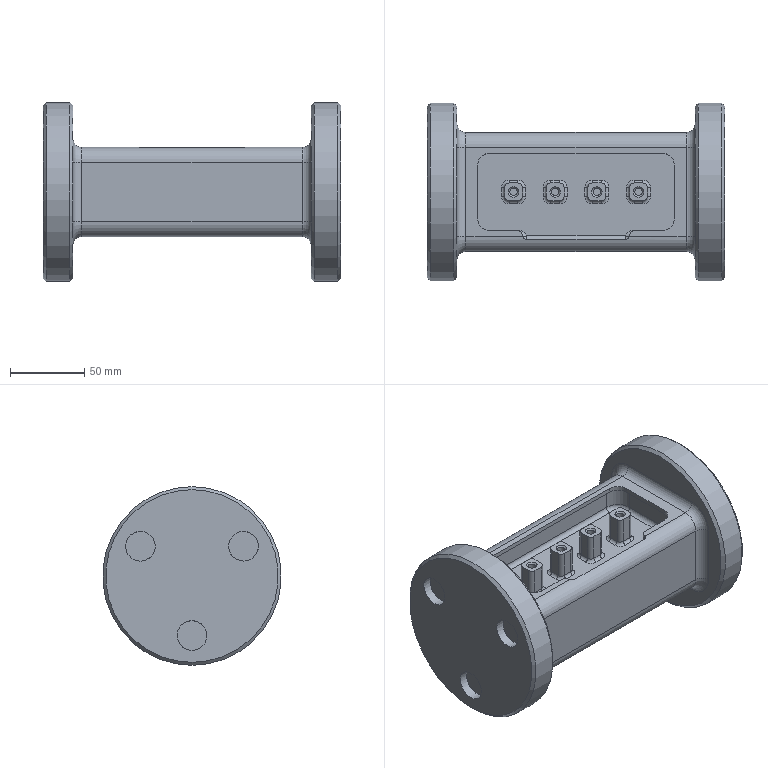NC program | NX | posted with a generic post | part box 200 x 120 x 120 mm
Lines 1229 to 3124 of 4340:
(ZLEVEL_PROFILE , TOOL : D10R1)
N2444 M6
N2446 G53
N2448 G17 G0 G90 X45. Y-16. S0 M3
N2450 G43 Z40. H0
N2452 Z-1.
N2454 G94 G1 Y-14. F250.
N2456 G3 X42. Y-11. R3.
N2458 G1 X39.
N2460 G2 X31. Y-3. R8.
N2462 G1 Y3.
N2464 G2 X39. Y11. R8.
N2466 G1 X45.
N2468 G2 X53. Y3. R8.
N2470 G1 Y-3.
N2472 G2 X45. Y-11. R8.
N2474 G1 X42.
N2476 Z-1.5
N2478 X39.
N2480 G2 X31. Y-3. R8.
N2482 G1 Y3.
N2484 G2 X39. Y11. R8.
N2486 G1 X45.
N2488 G2 X53. Y3. R8.
N2490 G1 Y-3.
N2492 G2 X45. Y-11. R8.
N2494 G1 X42.
N2496 Z-2.
N2498 X39.
N2500 G2 X31. Y-3. R8.
N2502 G1 Y3.
N2504 G2 X39. Y11. R8.
N2506 G1 X45.
N2508 G2 X53. Y3. R8.
N2510 G1 Y-3.
N2512 G2 X45. Y-11. R8.
N2514 G1 X42.
N2516 Z-2.5
N2518 X39.
N2520 G2 X31. Y-3. R8.
N2522 G1 Y3.
N2524 G2 X39. Y11. R8.
N2526 G1 X45.
N2528 G2 X53. Y3. R8.
N2530 G1 Y-3.
N2532 G2 X45. Y-11. R8.
N2534 G1 X42.
N2536 Z-3.
N2538 X39.
N2540 G2 X31. Y-3. R8.
N2542 G1 Y3.
N2544 G2 X39. Y11. R8.
N2546 G1 X45.
N2548 G2 X53. Y3. R8.
N2550 G1 Y-3.
N2552 G2 X45. Y-11. R8.
N2554 G1 X42.
N2556 Z-3.5
N2558 X39.
N2560 G2 X31. Y-3. R8.
N2562 G1 Y3.
N2564 G2 X39. Y11. R8.
N2566 G1 X45.
N2568 G2 X53. Y3. R8.
N2570 G1 Y-3.
N2572 G2 X45. Y-11. R8.
N2574 G1 X42.
N2576 Z-4.
N2578 X39.
N2580 G2 X31. Y-3. R8.
N2582 G1 Y3.
N2584 G2 X39. Y11. R8.
N2586 G1 X45.
N2588 G2 X53. Y3. R8.
N2590 G1 Y-3.
N2592 G2 X45. Y-11. R8.
N2594 G1 X42.
N2596 Z-4.5
N2598 X39.
N2600 G2 X31. Y-3. R8.
N2602 G1 Y3.
N2604 G2 X39. Y11. R8.
N2606 G1 X45.
N2608 G2 X53. Y3. R8.
N2610 G1 Y-3.
N2612 G2 X45. Y-11. R8.
N2614 G1 X42.
N2616 Z-5.
N2618 X39.
N2620 G2 X31. Y-3. R8.
N2622 G1 Y3.
N2624 G2 X39. Y11. R8.
N2626 G1 X45.
N2628 G2 X53. Y3. R8.
N2630 G1 Y-3.
N2632 G2 X45. Y-11. R8.
N2634 G1 X42.
N2636 Z-5.5
N2638 X39.
N2640 G2 X31. Y-3. R8.
N2642 G1 Y3.
N2644 G2 X39. Y11. R8.
N2646 G1 X45.
N2648 G2 X53. Y3. R8.
N2650 G1 Y-3.
N2652 G2 X45. Y-11. R8.
N2654 G1 X42.
N2656 Z-6.
N2658 X39.
N2660 G2 X31. Y-3. R8.
N2662 G1 Y3.
N2664 G2 X39. Y11. R8.
N2666 G1 X45.
N2668 G2 X53. Y3. R8.
N2670 G1 Y-3.
N2672 G2 X45. Y-11. R8.
N2674 G1 X42.
N2676 Z-6.5
N2678 X39.
N2680 G2 X31. Y-3. R8.
N2682 G1 Y3.
N2684 G2 X39. Y11. R8.
N2686 G1 X45.
N2688 G2 X53. Y3. R8.
N2690 G1 Y-3.
N2692 G2 X45. Y-11. R8.
N2694 G1 X42.
N2696 Z-7.
N2698 X39.
N2700 G2 X31. Y-3. R8.
N2702 G1 Y3.
N2704 G2 X39. Y11. R8.
N2706 G1 X45.
N2708 G2 X53. Y3. R8.
N2710 G1 Y-3.
N2712 G2 X45. Y-11. R8.
N2714 G1 X42.
N2716 Z-7.5
N2718 X39.
N2720 G2 X31. Y-3. R8.
N2722 G1 Y3.
N2724 G2 X39. Y11. R8.
N2726 G1 X45.
N2728 G2 X53. Y3. R8.
N2730 G1 Y-3.
N2732 G2 X45. Y-11. R8.
N2734 G1 X42.
N2736 Z-8.
N2738 X39.
N2740 G2 X31. Y-3. R8.
N2742 G1 Y3.
N2744 G2 X39. Y11. R8.
N2746 G1 X45.
N2748 G2 X53. Y3. R8.
N2750 G1 Y-3.
N2752 G2 X45. Y-11. R8.
N2754 G1 X42.
N2756 Z-8.5
N2758 X39.
N2760 G2 X31. Y-3. R8.
N2762 G1 Y3.
N2764 G2 X39. Y11. R8.
N2766 G1 X45.
N2768 G2 X53. Y3. R8.
N2770 G1 Y-3.
N2772 G2 X45. Y-11. R8.
N2774 G1 X42.
N2776 Z-9.
N2778 X39.
N2780 G2 X31. Y-3. R8.
N2782 G1 Y3.
N2784 G2 X39. Y11. R8.
N2786 G1 X45.
N2788 G2 X53. Y3. R8.
N2790 G1 Y-3.
N2792 G2 X45. Y-11. R8.
N2794 G1 X42.
N2796 Z-9.5
N2798 X39.
N2800 G2 X31. Y-3. R8.
N2802 G1 Y3.
N2804 G2 X39. Y11. R8.
N2806 G1 X45.
N2808 G2 X53. Y3. R8.
N2810 G1 Y-3.
N2812 G2 X45. Y-11. R8.
N2814 G1 X42.
N2816 Z-10.
N2818 X39.
N2820 G2 X31. Y-3. R8.
N2822 G1 Y3.
N2824 G2 X39. Y11. R8.
N2826 G1 X45.
N2828 G2 X53. Y3. R8.
N2830 G1 Y-3.
N2832 G2 X45. Y-11. R8.
N2834 G1 X42.
N2836 Z-10.5
N2838 X39.
N2840 G2 X31. Y-3. R8.
N2842 G1 Y3.
N2844 G2 X39. Y11. R8.
N2846 G1 X45.
N2848 G2 X53. Y3. R8.
N2850 G1 Y-3.
N2852 G2 X45. Y-11. R8.
N2854 G1 X42.
N2856 Z-11.
N2858 X39.
N2860 G2 X31. Y-3. R8.
N2862 G1 Y3.
N2864 G2 X39. Y11. R8.
N2866 G1 X45.
N2868 G2 X53. Y3. R8.
N2870 G1 Y-3.
N2872 G2 X45. Y-11. R8.
N2874 G1 X42.
N2876 Z-11.5
N2878 X39.
N2880 G2 X31. Y-3. R8.
N2882 G1 Y3.
N2884 G2 X39. Y11. R8.
N2886 G1 X45.
N2888 G2 X53. Y3. R8.
N2890 G1 Y-3.
N2892 G2 X45. Y-11. R8.
N2894 G1 X42.
N2896 Z-12.
N2898 X39.
N2900 G2 X31. Y-3. R8.
N2902 G1 Y3.
N2904 G2 X39. Y11. R8.
N2906 G1 X45.
N2908 G2 X53. Y3. R8.
N2910 G1 Y-3.
N2912 G2 X45. Y-11. R8.
N2914 G1 X42.
N2916 Z-12.5
N2918 X39.
N2920 G2 X31. Y-3. R8.
N2922 G1 Y3.
N2924 G2 X39. Y11. R8.
N2926 G1 X45.
N2928 G2 X53. Y3. R8.
N2930 G1 Y-3.
N2932 G2 X45. Y-11. R8.
N2934 G1 X42.
N2936 Z-13.
N2938 X39.
N2940 G2 X31. Y-3. R8.
N2942 G1 Y3.
N2944 G2 X39. Y11. R8.
N2946 G1 X45.
N2948 G2 X53. Y3. R8.
N2950 G1 Y-3.
N2952 G2 X45. Y-11. R8.
N2954 G1 X42.
N2956 Z-13.5
N2958 X39.
N2960 G2 X31. Y-3. R8.
N2962 G1 Y3.
N2964 G2 X39. Y11. R8.
N2966 G1 X45.
N2968 G2 X53. Y3. R8.
N2970 G1 Y-3.
N2972 G2 X45. Y-11. R8.
N2974 G1 X42.
N2976 Z-14.
N2978 X39.
N2980 G2 X31. Y-3. R8.
N2982 G1 Y3.
N2984 G2 X39. Y11. R8.
N2986 G1 X45.
N2988 G2 X53. Y3. R8.
N2990 G1 Y-3.
N2992 G2 X45. Y-11. R8.
N2994 G1 X42.
N2996 Z-14.5
N2998 X39.
N3000 G2 X31. Y-3. R8.
N3002 G1 Y3.
N3004 G2 X39. Y11. R8.
N3006 G1 X45.
N3008 G2 X53. Y3. R8.
N3010 G1 Y-3.
N3012 G2 X45. Y-11. R8.
N3014 G1 X42.
N3016 Z-15.
N3018 X39.
N3020 G2 X31. Y-3. R8.
N3022 G1 Y3.
N3024 G2 X39. Y11. R8.
N3026 G1 X45.
N3028 G2 X53. Y3. R8.
N3030 G1 Y-3.
N3032 G2 X45. Y-11. R8.
N3034 G1 X42.
N3036 Z-15.5
N3038 X39.
N3040 G2 X31. Y-3. R8.
N3042 G1 Y3.
N3044 G2 X39. Y11. R8.
N3046 G1 X45.
N3048 G2 X53. Y3. R8.
N3050 G1 Y-3.
N3052 G2 X45. Y-11. R8.
N3054 G1 X42.
N3056 Z-16.
N3058 X39.
N3060 G2 X31. Y-3. R8.
N3062 G1 Y3.
N3064 G2 X39. Y11. R8.
N3066 G1 X45.
N3068 G2 X53. Y3. R8.
N3070 G1 Y-3.
N3072 G2 X45. Y-11. R8.
N3074 G1 X42.
N3076 Z-16.5
N3078 X39.
N3080 G2 X31. Y-3. R8.
N3082 G1 Y3.
N3084 G2 X39. Y11. R8.
N3086 G1 X45.
N3088 G2 X53. Y3. R8.
N3090 G1 Y-3.
N3092 G2 X45. Y-11. R8.
N3094 G1 X42.
N3096 Z-17.
N3098 X39.
N3100 G2 X31. Y-3. R8.
N3102 G1 Y3.
N3104 G2 X39. Y11. R8.
N3106 G1 X45.
N3108 G2 X53. Y3. R8.
N3110 G1 Y-3.
N3112 G2 X45. Y-11. R8.
N3114 G1 X42.
N3116 Z-17.5
N3118 X39.
N3120 G2 X31. Y-3. R8.
N3122 G1 Y3.
N3124 G2 X39. Y11. R8.
N3126 G1 X45.
N3128 G2 X53. Y3. R8.
N3130 G1 Y-3.
N3132 G2 X45. Y-11. R8.
N3134 G1 X42.
N3136 Z-18.
N3138 X39.
N3140 G2 X31. Y-3. R8.
N3142 G1 Y3.
N3144 G2 X39. Y11. R8.
N3146 G1 X45.
N3148 G2 X53. Y3. R8.
N3150 G1 Y-3.
N3152 G2 X45. Y-11. R8.
N3154 G1 X42.
N3156 Z-18.5
N3158 X39.
N3160 G2 X31. Y-3. R8.
N3162 G1 Y3.
N3164 G2 X39. Y11. R8.
N3166 G1 X45.
N3168 G2 X53. Y3. R8.
N3170 G1 Y-3.
N3172 G2 X45. Y-11. R8.
N3174 G1 X42.
N3176 Z-19.
N3178 X39.
N3180 G2 X31. Y-3. R8.
N3182 G1 Y3.
N3184 G2 X39. Y11. R8.
N3186 G1 X45.
N3188 G2 X53. Y3. R8.
N3190 G1 Y-3.
N3192 G2 X45. Y-11. R8.
N3194 G1 X42.
N3196 Y-11.008 Z-19.125
N3198 Y-11.032 Z-19.25
N3200 Y-11.073 Z-19.375
N3202 Y-11.134 Z-19.5
N3204 X39.
N3206 G2 X30.866 Y-3. R8.134
N3208 G1 Y3.
N3210 G2 X39. Y11.134 R8.134
N3212 G1 X45.
N3214 G2 X53.134 Y3. R8.134
N3216 G1 Y-3.
N3218 G2 X45. Y-11.134 R8.134
N3220 G1 X42.
N3222 Y-11.219 Z-19.625
N3224 Y-11.339 Z-19.75
N3226 Y-11.417 Z-19.813
N3228 Y-11.516 Z-19.875
N3230 Y-11.652 Z-19.938
N3232 Y-11.878 Z-20.
N3234 X39.
N3236 G2 X30.122 Y-3. R8.878
N3238 G1 Y3.
N3240 G2 X39. Y11.878 R8.878
N3242 G1 X45.
N3244 G2 X53.878 Y3. R8.878
N3246 G1 Y-3.
N3248 G2 X45. Y-11.878 R8.878
N3250 G1 X42.
N3252 G3 X39. Y-14.878 R3.
N3254 G1 Y-16.878
N3256 G0 Z40.
N3258 X17. Y-16.
N3260 Z-1.
N3262 G1 Y-14.
N3264 G3 X14. Y-11. R3.
N3266 G1 X11.
N3268 G2 X3. Y-3. R8.
N3270 G1 Y3.
N3272 G2 X11. Y11. R8.
N3274 G1 X17.
N3276 G2 X25. Y3. R8.
N3278 G1 Y-3.
N3280 G2 X17. Y-11. R8.
N3282 G1 X14.
N3284 Z-1.5
N3286 X11.
N3288 G2 X3. Y-3. R8.
N3290 G1 Y3.
N3292 G2 X11. Y11. R8.
N3294 G1 X17.
N3296 G2 X25. Y3. R8.
N3298 G1 Y-3.
N3300 G2 X17. Y-11. R8.
N3302 G1 X14.
N3304 Z-2.
N3306 X11.
N3308 G2 X3. Y-3. R8.
N3310 G1 Y3.
N3312 G2 X11. Y11. R8.
N3314 G1 X17.
N3316 G2 X25. Y3. R8.
N3318 G1 Y-3.
N3320 G2 X17. Y-11. R8.
N3322 G1 X14.
N3324 Z-2.5
N3326 X11.
N3328 G2 X3. Y-3. R8.
N3330 G1 Y3.
N3332 G2 X11. Y11. R8.
N3334 G1 X17.
N3336 G2 X25. Y3. R8.
N3338 G1 Y-3.
N3340 G2 X17. Y-11. R8.
N3342 G1 X14.
N3344 Z-3.
N3346 X11.
N3348 G2 X3. Y-3. R8.
N3350 G1 Y3.
N3352 G2 X11. Y11. R8.
N3354 G1 X17.
N3356 G2 X25. Y3. R8.
N3358 G1 Y-3.
N3360 G2 X17. Y-11. R8.
N3362 G1 X14.
N3364 Z-3.5
N3366 X11.
N3368 G2 X3. Y-3. R8.
N3370 G1 Y3.
N3372 G2 X11. Y11. R8.
N3374 G1 X17.
N3376 G2 X25. Y3. R8.
N3378 G1 Y-3.
N3380 G2 X17. Y-11. R8.
N3382 G1 X14.
N3384 Z-4.
N3386 X11.
N3388 G2 X3. Y-3. R8.
N3390 G1 Y3.
N3392 G2 X11. Y11. R8.
N3394 G1 X17.
N3396 G2 X25. Y3. R8.
N3398 G1 Y-3.
N3400 G2 X17. Y-11. R8.
N3402 G1 X14.
N3404 Z-4.5
N3406 X11.
N3408 G2 X3. Y-3. R8.
N3410 G1 Y3.
N3412 G2 X11. Y11. R8.
N3414 G1 X17.
N3416 G2 X25. Y3. R8.
N3418 G1 Y-3.
N3420 G2 X17. Y-11. R8.
N3422 G1 X14.
N3424 Z-5.
N3426 X11.
N3428 G2 X3. Y-3. R8.
N3430 G1 Y3.
N3432 G2 X11. Y11. R8.
N3434 G1 X17.
N3436 G2 X25. Y3. R8.
N3438 G1 Y-3.
N3440 G2 X17. Y-11. R8.
N3442 G1 X14.
N3444 Z-5.5
N3446 X11.
N3448 G2 X3. Y-3. R8.
N3450 G1 Y3.
N3452 G2 X11. Y11. R8.
N3454 G1 X17.
N3456 G2 X25. Y3. R8.
N3458 G1 Y-3.
N3460 G2 X17. Y-11. R8.
N3462 G1 X14.
N3464 Z-6.
N3466 X11.
N3468 G2 X3. Y-3. R8.
N3470 G1 Y3.
N3472 G2 X11. Y11. R8.
N3474 G1 X17.
N3476 G2 X25. Y3. R8.
N3478 G1 Y-3.
N3480 G2 X17. Y-11. R8.
N3482 G1 X14.
N3484 Z-6.5
N3486 X11.
N3488 G2 X3. Y-3. R8.
N3490 G1 Y3.
N3492 G2 X11. Y11. R8.
N3494 G1 X17.
N3496 G2 X25. Y3. R8.
N3498 G1 Y-3.
N3500 G2 X17. Y-11. R8.
N3502 G1 X14.
N3504 Z-7.
N3506 X11.
N3508 G2 X3. Y-3. R8.
N3510 G1 Y3.
N3512 G2 X11. Y11. R8.
N3514 G1 X17.
N3516 G2 X25. Y3. R8.
N3518 G1 Y-3.
N3520 G2 X17. Y-11. R8.
N3522 G1 X14.
N3524 Z-7.5
N3526 X11.
N3528 G2 X3. Y-3. R8.
N3530 G1 Y3.
N3532 G2 X11. Y11. R8.
N3534 G1 X17.
N3536 G2 X25. Y3. R8.
N3538 G1 Y-3.
N3540 G2 X17. Y-11. R8.
N3542 G1 X14.
N3544 Z-8.
N3546 X11.
N3548 G2 X3. Y-3. R8.
N3550 G1 Y3.
N3552 G2 X11. Y11. R8.
N3554 G1 X17.
N3556 G2 X25. Y3. R8.
N3558 G1 Y-3.
N3560 G2 X17. Y-11. R8.
N3562 G1 X14.
N3564 Z-8.5
N3566 X11.
N3568 G2 X3. Y-3. R8.
N3570 G1 Y3.
N3572 G2 X11. Y11. R8.
N3574 G1 X17.
N3576 G2 X25. Y3. R8.
N3578 G1 Y-3.
N3580 G2 X17. Y-11. R8.
N3582 G1 X14.
N3584 Z-9.
N3586 X11.
N3588 G2 X3. Y-3. R8.
N3590 G1 Y3.
N3592 G2 X11. Y11. R8.
N3594 G1 X17.
N3596 G2 X25. Y3. R8.
N3598 G1 Y-3.
N3600 G2 X17. Y-11. R8.
N3602 G1 X14.
N3604 Z-9.5
N3606 X11.
N3608 G2 X3. Y-3. R8.
N3610 G1 Y3.
N3612 G2 X11. Y11. R8.
N3614 G1 X17.
N3616 G2 X25. Y3. R8.
N3618 G1 Y-3.
N3620 G2 X17. Y-11. R8.
N3622 G1 X14.
N3624 Z-10.
N3626 X11.
N3628 G2 X3. Y-3. R8.
N3630 G1 Y3.
N3632 G2 X11. Y11. R8.
N3634 G1 X17.
N3636 G2 X25. Y3. R8.
N3638 G1 Y-3.
N3640 G2 X17. Y-11. R8.
N3642 G1 X14.
N3644 Z-10.5
N3646 X11.
N3648 G2 X3. Y-3. R8.
N3650 G1 Y3.
N3652 G2 X11. Y11. R8.
N3654 G1 X17.
N3656 G2 X25. Y3. R8.
N3658 G1 Y-3.
N3660 G2 X17. Y-11. R8.
N3662 G1 X14.
N3664 Z-11.
N3666 X11.
N3668 G2 X3. Y-3. R8.
N3670 G1 Y3.
N3672 G2 X11. Y11. R8.
N3674 G1 X17.
N3676 G2 X25. Y3. R8.
N3678 G1 Y-3.
N3680 G2 X17. Y-11. R8.
N3682 G1 X14.
N3684 Z-11.5
N3686 X11.
N3688 G2 X3. Y-3. R8.
N3690 G1 Y3.
N3692 G2 X11. Y11. R8.
N3694 G1 X17.
N3696 G2 X25. Y3. R8.
N3698 G1 Y-3.
N3700 G2 X17. Y-11. R8.
N3702 G1 X14.
N3704 Z-12.
N3706 X11.
N3708 G2 X3. Y-3. R8.
N3710 G1 Y3.
N3712 G2 X11. Y11. R8.
N3714 G1 X17.
N3716 G2 X25. Y3. R8.
N3718 G1 Y-3.
N3720 G2 X17. Y-11. R8.
N3722 G1 X14.
N3724 Z-12.5
N3726 X11.
N3728 G2 X3. Y-3. R8.
N3730 G1 Y3.
N3732 G2 X11. Y11. R8.
N3734 G1 X17.
N3736 G2 X25. Y3. R8.
N3738 G1 Y-3.
N3740 G2 X17. Y-11. R8.
N3742 G1 X14.
N3744 Z-13.
N3746 X11.
N3748 G2 X3. Y-3. R8.
N3750 G1 Y3.
N3752 G2 X11. Y11. R8.
N3754 G1 X17.
N3756 G2 X25. Y3. R8.
N3758 G1 Y-3.
N3760 G2 X17. Y-11. R8.
N3762 G1 X14.
N3764 Z-13.5
N3766 X11.
N3768 G2 X3. Y-3. R8.
N3770 G1 Y3.
N3772 G2 X11. Y11. R8.
N3774 G1 X17.
N3776 G2 X25. Y3. R8.
N3778 G1 Y-3.
N3780 G2 X17. Y-11. R8.
N3782 G1 X14.
N3784 Z-14.
N3786 X11.
N3788 G2 X3. Y-3. R8.
N3790 G1 Y3.
N3792 G2 X11. Y11. R8.
N3794 G1 X17.
N3796 G2 X25. Y3. R8.
N3798 G1 Y-3.
N3800 G2 X17. Y-11. R8.
N3802 G1 X14.
N3804 Z-14.5
N3806 X11.
N3808 G2 X3. Y-3. R8.
N3810 G1 Y3.
N3812 G2 X11. Y11. R8.
N3814 G1 X17.
N3816 G2 X25. Y3. R8.
N3818 G1 Y-3.
N3820 G2 X17. Y-11. R8.
N3822 G1 X14.
N3824 Z-15.
N3826 X11.
N3828 G2 X3. Y-3. R8.
N3830 G1 Y3.
N3832 G2 X11. Y11. R8.
N3834 G1 X17.
N3836 G2 X25. Y3. R8.
N3838 G1 Y-3.
N3840 G2 X17. Y-11. R8.
N3842 G1 X14.
N3844 Z-15.5
N3846 X11.
N3848 G2 X3. Y-3. R8.
N3850 G1 Y3.
N3852 G2 X11. Y11. R8.
N3854 G1 X17.
N3856 G2 X25. Y3. R8.
N3858 G1 Y-3.
N3860 G2 X17. Y-11. R8.
N3862 G1 X14.
N3864 Z-16.
N3866 X11.
N3868 G2 X3. Y-3. R8.
N3870 G1 Y3.
N3872 G2 X11. Y11. R8.
N3874 G1 X17.
N3876 G2 X25. Y3. R8.
N3878 G1 Y-3.
N3880 G2 X17. Y-11. R8.
N3882 G1 X14.
N3884 Z-16.5
N3886 X11.
N3888 G2 X3. Y-3. R8.
N3890 G1 Y3.
N3892 G2 X11. Y11. R8.
N3894 G1 X17.
N3896 G2 X25. Y3. R8.
N3898 G1 Y-3.
N3900 G2 X17. Y-11. R8.
N3902 G1 X14.
N3904 Z-17.
N3906 X11.
N3908 G2 X3. Y-3. R8.
N3910 G1 Y3.
N3912 G2 X11. Y11. R8.
N3914 G1 X17.
N3916 G2 X25. Y3. R8.
N3918 G1 Y-3.
N3920 G2 X17. Y-11. R8.
N3922 G1 X14.
N3924 Z-17.5
N3926 X11.
N3928 G2 X3. Y-3. R8.
N3930 G1 Y3.
N3932 G2 X11. Y11. R8.
N3934 G1 X17.
N3936 G2 X25. Y3. R8.
N3938 G1 Y-3.
N3940 G2 X17. Y-11. R8.
N3942 G1 X14.
N3944 Z-18.
N3946 X11.
N3948 G2 X3. Y-3. R8.
N3950 G1 Y3.
N3952 G2 X11. Y11. R8.
N3954 G1 X17.
N3956 G2 X25. Y3. R8.
N3958 G1 Y-3.
N3960 G2 X17. Y-11. R8.
N3962 G1 X14.
N3964 Z-18.5
N3966 X11.
N3968 G2 X3. Y-3. R8.
N3970 G1 Y3.
N3972 G2 X11. Y11. R8.
N3974 G1 X17.
N3976 G2 X25. Y3. R8.
N3978 G1 Y-3.
N3980 G2 X17. Y-11. R8.
N3982 G1 X14.
N3984 Z-19.
N3986 X11.
N3988 G2 X3. Y-3. R8.
N3990 G1 Y3.
N3992 G2 X11. Y11. R8.
N3994 G1 X17.
N3996 G2 X25. Y3. R8.
N3998 G1 Y-3.
N4000 G2 X17. Y-11. R8.
N4002 G1 X14.
N4004 Y-11.008 Z-19.125
N4006 Y-11.032 Z-19.25
N4008 Y-11.073 Z-19.375
N4010 Y-11.134 Z-19.5
N4012 X11.
N4014 G2 X2.866 Y-3. R8.134
N4016 G1 Y3.
N4018 G2 X11. Y11.134 R8.134
N4020 G1 X17.
N4022 G2 X25.134 Y3. R8.134
N4024 G1 Y-3.
N4026 G2 X17. Y-11.134 R8.134
N4028 G1 X14.
N4030 Y-11.219 Z-19.625
N4032 Y-11.339 Z-19.75
N4034 Y-11.417 Z-19.813
N4036 Y-11.516 Z-19.875
N4038 Y-11.652 Z-19.938
N4040 Y-11.878 Z-20.
N4042 X11.
N4044 G2 X2.122 Y-3. R8.878
N4046 G1 Y3.
N4048 G2 X11. Y11.878 R8.878
N4050 G1 X17.
N4052 G2 X25.878 Y3. R8.878
N4054 G1 Y-3.
N4056 G2 X17. Y-11.878 R8.878
N4058 G1 X14.
N4060 G3 X11. Y-14.878 R3.
N4062 G1 Y-16.878
N4064 G0 Z40.
N4066 X-11. Y-16.
N4068 Z-1.
N4070 G1 Y-14.
N4072 G3 X-14. Y-11. R3.
N4074 G1 X-17.
N4076 G2 X-25. Y-3. R8.
N4078 G1 Y3.
N4080 G2 X-17. Y11. R8.
N4082 G1 X-11.
N4084 G2 X-3. Y3. R8.
N4086 G1 Y-3.
N4088 G2 X-11. Y-11. R8.
N4090 G1 X-14.
N4092 Z-1.5
N4094 X-17.
N4096 G2 X-25. Y-3. R8.
N4098 G1 Y3.
N4100 G2 X-17. Y11. R8.
N4102 G1 X-11.
N4104 G2 X-3. Y3. R8.
N4106 G1 Y-3.
N4108 G2 X-11. Y-11. R8.
N4110 G1 X-14.
N4112 Z-2.
N4114 X-17.
N4116 G2 X-25. Y-3. R8.
N4118 G1 Y3.
N4120 G2 X-17. Y11. R8.
N4122 G1 X-11.
N4124 G2 X-3. Y3. R8.
N4126 G1 Y-3.
N4128 G2 X-11. Y-11. R8.
N4130 G1 X-14.
N4132 Z-2.5
N4134 X-17.
N4136 G2 X-25. Y-3. R8.
N4138 G1 Y3.
N4140 G2 X-17. Y11. R8.
N4142 G1 X-11.
N4144 G2 X-3. Y3. R8.
N4146 G1 Y-3.
N4148 G2 X-11. Y-11. R8.
N4150 G1 X-14.
N4152 Z-3.
N4154 X-17.
N4156 G2 X-25. Y-3. R8.
N4158 G1 Y3.
N4160 G2 X-17. Y11. R8.
N4162 G1 X-11.
N4164 G2 X-3. Y3. R8.
N4166 G1 Y-3.
N4168 G2 X-11. Y-11. R8.
N4170 G1 X-14.
N4172 Z-3.5
N4174 X-17.
N4176 G2 X-25. Y-3. R8.
N4178 G1 Y3.
N4180 G2 X-17. Y11. R8.
N4182 G1 X-11.
N4184 G2 X-3. Y3. R8.
N4186 G1 Y-3.
N4188 G2 X-11. Y-11. R8.
N4190 G1 X-14.
N4192 Z-4.
N4194 X-17.
N4196 G2 X-25. Y-3. R8.
N4198 G1 Y3.
N4200 G2 X-17. Y11. R8.
N4202 G1 X-11.
N4204 G2 X-3. Y3. R8.
N4206 G1 Y-3.
N4208 G2 X-11. Y-11. R8.
N4210 G1 X-14.
N4212 Z-4.5
N4214 X-17.
N4216 G2 X-25. Y-3. R8.
N4218 G1 Y3.
N4220 G2 X-17. Y11. R8.
N4222 G1 X-11.
N4224 G2 X-3. Y3. R8.
N4226 G1 Y-3.
N4228 G2 X-11. Y-11. R8.
N4230 G1 X-14.
N4232 Z-5.
N4234 X-17.
N4236 G2 X-25. Y-3. R8.
N4238 G1 Y3.
N4240 G2 X-17. Y11. R8.
N4242 G1 X-11.
N4244 G2 X-3. Y3. R8.
N4246 G1 Y-3.
N4248 G2 X-11. Y-11. R8.
N4250 G1 X-14.
N4252 Z-5.5
N4254 X-17.
N4256 G2 X-25. Y-3. R8.
N4258 G1 Y3.
N4260 G2 X-17. Y11. R8.
N4262 G1 X-11.
N4264 G2 X-3. Y3. R8.
N4266 G1 Y-3.
N4268 G2 X-11. Y-11. R8.
N4270 G1 X-14.
N4272 Z-6.
N4274 X-17.
N4276 G2 X-25. Y-3. R8.
N4278 G1 Y3.
N4280 G2 X-17. Y11. R8.
N4282 G1 X-11.
N4284 G2 X-3. Y3. R8.
N4286 G1 Y-3.
N4288 G2 X-11. Y-11. R8.
N4290 G1 X-14.
N4292 Z-6.5
N4294 X-17.
N4296 G2 X-25. Y-3. R8.
N4298 G1 Y3.
N4300 G2 X-17. Y11. R8.
N4302 G1 X-11.
N4304 G2 X-3. Y3. R8.
N4306 G1 Y-3.
N4308 G2 X-11. Y-11. R8.
N4310 G1 X-14.
N4312 Z-7.
N4314 X-17.
N4316 G2 X-25. Y-3. R8.
N4318 G1 Y3.
N4320 G2 X-17. Y11. R8.
N4322 G1 X-11.
N4324 G2 X-3. Y3. R8.
N4326 G1 Y-3.
N4328 G2 X-11. Y-11. R8.
N4330 G1 X-14.
N4332 Z-7.5
N4334 X-17.
N4336 G2 X-25. Y-3. R8.
N4338 G1 Y3.
N4340 G2 X-17. Y11. R8.
N4342 G1 X-11.
N4344 G2 X-3. Y3. R8.
N4346 G1 Y-3.
N4348 G2 X-11. Y-11. R8.
N4350 G1 X-14.
N4352 Z-8.
N4354 X-17.
N4356 G2 X-25. Y-3. R8.
N4358 G1 Y3.
N4360 G2 X-17. Y11. R8.
N4362 G1 X-11.
N4364 G2 X-3. Y3. R8.
N4366 G1 Y-3.
N4368 G2 X-11. Y-11. R8.
N4370 G1 X-14.
N4372 Z-8.5
N4374 X-17.
N4376 G2 X-25. Y-3. R8.
N4378 G1 Y3.
N4380 G2 X-17. Y11. R8.
N4382 G1 X-11.
N4384 G2 X-3. Y3. R8.
N4386 G1 Y-3.
N4388 G2 X-11. Y-11. R8.
N4390 G1 X-14.
N4392 Z-9.
N4394 X-17.
N4396 G2 X-25. Y-3. R8.
N4398 G1 Y3.
N4400 G2 X-17. Y11. R8.
N4402 G1 X-11.
N4404 G2 X-3. Y3. R8.
N4406 G1 Y-3.
N4408 G2 X-11. Y-11. R8.
N4410 G1 X-14.
N4412 Z-9.5
N4414 X-17.
N4416 G2 X-25. Y-3. R8.
N4418 G1 Y3.
N4420 G2 X-17. Y11. R8.
N4422 G1 X-11.
N4424 G2 X-3. Y3. R8.
N4426 G1 Y-3.
N4428 G2 X-11. Y-11. R8.
N4430 G1 X-14.
N4432 Z-10.
N4434 X-17.
N4436 G2 X-25. Y-3. R8.
N4438 G1 Y3.
N4440 G2 X-17. Y11. R8.
N4442 G1 X-11.
N4444 G2 X-3. Y3. R8.
N4446 G1 Y-3.
N4448 G2 X-11. Y-11. R8.
N4450 G1 X-14.
N4452 Z-10.5
N4454 X-17.
N4456 G2 X-25. Y-3. R8.
N4458 G1 Y3.
N4460 G2 X-17. Y11. R8.
N4462 G1 X-11.
N4464 G2 X-3. Y3. R8.
N4466 G1 Y-3.
N4468 G2 X-11. Y-11. R8.
N4470 G1 X-14.
N4472 Z-11.
N4474 X-17.
N4476 G2 X-25. Y-3. R8.
N4478 G1 Y3.
N4480 G2 X-17. Y11. R8.
N4482 G1 X-11.
N4484 G2 X-3. Y3. R8.
N4486 G1 Y-3.
N4488 G2 X-11. Y-11. R8.
N4490 G1 X-14.
N4492 Z-11.5
N4494 X-17.
N4496 G2 X-25. Y-3. R8.
N4498 G1 Y3.
N4500 G2 X-17. Y11. R8.
N4502 G1 X-11.
N4504 G2 X-3. Y3. R8.
N4506 G1 Y-3.
N4508 G2 X-11. Y-11. R8.
N4510 G1 X-14.
N4512 Z-12.
N4514 X-17.
N4516 G2 X-25. Y-3. R8.
N4518 G1 Y3.
N4520 G2 X-17. Y11. R8.
N4522 G1 X-11.
N4524 G2 X-3. Y3. R8.
N4526 G1 Y-3.
N4528 G2 X-11. Y-11. R8.
N4530 G1 X-14.
N4532 Z-12.5
N4534 X-17.
N4536 G2 X-25. Y-3. R8.
N4538 G1 Y3.
N4540 G2 X-17. Y11. R8.
N4542 G1 X-11.
N4544 G2 X-3. Y3. R8.
N4546 G1 Y-3.
N4548 G2 X-11. Y-11. R8.
N4550 G1 X-14.
N4552 Z-13.
N4554 X-17.
N4556 G2 X-25. Y-3. R8.
N4558 G1 Y3.
N4560 G2 X-17. Y11. R8.
N4562 G1 X-11.
N4564 G2 X-3. Y3. R8.
N4566 G1 Y-3.
N4568 G2 X-11. Y-11. R8.
N4570 G1 X-14.
N4572 Z-13.5
N4574 X-17.
N4576 G2 X-25. Y-3. R8.
N4578 G1 Y3.
N4580 G2 X-17. Y11. R8.
N4582 G1 X-11.
N4584 G2 X-3. Y3. R8.
N4586 G1 Y-3.
N4588 G2 X-11. Y-11. R8.
N4590 G1 X-14.
N4592 Z-14.
N4594 X-17.
N4596 G2 X-25. Y-3. R8.
N4598 G1 Y3.
N4600 G2 X-17. Y11. R8.
N4602 G1 X-11.
N4604 G2 X-3. Y3. R8.
N4606 G1 Y-3.
N4608 G2 X-11. Y-11. R8.
N4610 G1 X-14.
N4612 Z-14.5
N4614 X-17.
N4616 G2 X-25. Y-3. R8.
N4618 G1 Y3.
N4620 G2 X-17. Y11. R8.
N4622 G1 X-11.
N4624 G2 X-3. Y3. R8.
N4626 G1 Y-3.
N4628 G2 X-11. Y-11. R8.
N4630 G1 X-14.
N4632 Z-15.
N4634 X-17.
N4636 G2 X-25. Y-3. R8.
N4638 G1 Y3.
N4640 G2 X-17. Y11. R8.
N4642 G1 X-11.
N4644 G2 X-3. Y3. R8.
N4646 G1 Y-3.
N4648 G2 X-11. Y-11. R8.
N4650 G1 X-14.
N4652 Z-15.5
N4654 X-17.
N4656 G2 X-25. Y-3. R8.
N4658 G1 Y3.
N4660 G2 X-17. Y11. R8.
N4662 G1 X-11.
N4664 G2 X-3. Y3. R8.
N4666 G1 Y-3.
N4668 G2 X-11. Y-11. R8.
N4670 G1 X-14.
N4672 Z-16.
N4674 X-17.
N4676 G2 X-25. Y-3. R8.
N4678 G1 Y3.
N4680 G2 X-17. Y11. R8.
N4682 G1 X-11.
N4684 G2 X-3. Y3. R8.
N4686 G1 Y-3.
N4688 G2 X-11. Y-11. R8.
N4690 G1 X-14.
N4692 Z-16.5
N4694 X-17.
N4696 G2 X-25. Y-3. R8.
N4698 G1 Y3.
N4700 G2 X-17. Y11. R8.
N4702 G1 X-11.
N4704 G2 X-3. Y3. R8.
N4706 G1 Y-3.
N4708 G2 X-11. Y-11. R8.
N4710 G1 X-14.
N4712 Z-17.
N4714 X-17.
N4716 G2 X-25. Y-3. R8.
N4718 G1 Y3.
N4720 G2 X-17. Y11. R8.
N4722 G1 X-11.
N4724 G2 X-3. Y3. R8.
N4726 G1 Y-3.
N4728 G2 X-11. Y-11. R8.
N4730 G1 X-14.
N4732 Z-17.5
N4734 X-17.
N4736 G2 X-25. Y-3. R8.
N4738 G1 Y3.
N4740 G2 X-17. Y11. R8.
N4742 G1 X-11.
N4744 G2 X-3. Y3. R8.
N4746 G1 Y-3.
N4748 G2 X-11. Y-11. R8.
N4750 G1 X-14.
N4752 Z-18.
N4754 X-17.
N4756 G2 X-25. Y-3. R8.
N4758 G1 Y3.
N4760 G2 X-17. Y11. R8.
N4762 G1 X-11.
N4764 G2 X-3. Y3. R8.
N4766 G1 Y-3.
N4768 G2 X-11. Y-11. R8.
N4770 G1 X-14.
N4772 Z-18.5
N4774 X-17.
N4776 G2 X-25. Y-3. R8.
N4778 G1 Y3.
N4780 G2 X-17. Y11. R8.
N4782 G1 X-11.
N4784 G2 X-3. Y3. R8.
N4786 G1 Y-3.
N4788 G2 X-11. Y-11. R8.
N4790 G1 X-14.
N4792 Z-19.
N4794 X-17.
N4796 G2 X-25. Y-3. R8.
N4798 G1 Y3.
N4800 G2 X-17. Y11. R8.
N4802 G1 X-11.
N4804 G2 X-3. Y3. R8.
N4806 G1 Y-3.
N4808 G2 X-11. Y-11. R8.
N4810 G1 X-14.
N4812 Y-11.008 Z-19.125
N4814 Y-11.032 Z-19.25
N4816 Y-11.073 Z-19.375
N4818 Y-11.134 Z-19.5
N4820 X-17.
N4822 G2 X-25.134 Y-3. R8.134
N4824 G1 Y3.
N4826 G2 X-17. Y11.134 R8.134
N4828 G1 X-11.
N4830 G2 X-2.866 Y3. R8.134
N4832 G1 Y-3.
N4834 G2 X-11. Y-11.134 R8.134
N4836 G1 X-14.
N4838 Y-11.219 Z-19.625
N4840 Y-11.339 Z-19.75
N4842 Y-11.417 Z-19.813
N4844 Y-11.516 Z-19.875
N4846 Y-11.652 Z-19.938
N4848 Y-11.878 Z-20.
N4850 X-17.
N4852 G2 X-25.878 Y-3. R8.878
N4854 G1 Y3.
N4856 G2 X-17. Y11.878 R8.878
N4858 G1 X-11.
N4860 G2 X-2.122 Y3. R8.878
N4862 G1 Y-3.
N4864 G2 X-11. Y-11.878 R8.878
N4866 G1 X-14.
N4868 G3 X-17. Y-14.878 R3.
N4870 G1 Y-16.878
N4872 G0 Z40.
N4874 X-39. Y-16.
N4876 Z-1.
N4878 G1 Y-14.
N4880 G3 X-42. Y-11. R3.
N4882 G1 X-45.
N4884 G2 X-53. Y-3. R8.
N4886 G1 Y3.
N4888 G2 X-45. Y11. R8.
N4890 G1 X-39.
N4892 G2 X-31. Y3. R8.
N4894 G1 Y-3.
N4896 G2 X-39. Y-11. R8.
N4898 G1 X-42.
N4900 Z-1.5
N4902 X-45.
N4904 G2 X-53. Y-3. R8.
N4906 G1 Y3.
N4908 G2 X-45. Y11. R8.
N4910 G1 X-39.
N4912 G2 X-31. Y3. R8.
N4914 G1 Y-3.
N4916 G2 X-39. Y-11. R8.
N4918 G1 X-42.
N4920 Z-2.
N4922 X-45.
N4924 G2 X-53. Y-3. R8.
N4926 G1 Y3.
N4928 G2 X-45. Y11. R8.
N4930 G1 X-39.
N4932 G2 X-31. Y3. R8.
N4934 G1 Y-3.
N4936 G2 X-39. Y-11. R8.
N4938 G1 X-42.
N4940 Z-2.5
N4942 X-45.
N4944 G2 X-53. Y-3. R8.
N4946 G1 Y3.
N4948 G2 X-45. Y11. R8.
N4950 G1 X-39.
N4952 G2 X-31. Y3. R8.
N4954 G1 Y-3.
N4956 G2 X-39. Y-11. R8.
N4958 G1 X-42.
N4960 Z-3.
N4962 X-45.
N4964 G2 X-53. Y-3. R8.
N4966 G1 Y3.
N4968 G2 X-45. Y11. R8.
N4970 G1 X-39.
N4972 G2 X-31. Y3. R8.
N4974 G1 Y-3.
N4976 G2 X-39. Y-11. R8.
N4978 G1 X-42.
N4980 Z-3.5
N4982 X-45.
N4984 G2 X-53. Y-3. R8.
N4986 G1 Y3.
N4988 G2 X-45. Y11. R8.
N4990 G1 X-39.
N4992 G2 X-31. Y3. R8.
N4994 G1 Y-3.
N4996 G2 X-39. Y-11. R8.
N4998 G1 X-42.
N5000 Z-4.
N5002 X-45.
N5004 G2 X-53. Y-3. R8.
N5006 G1 Y3.
N5008 G2 X-45. Y11. R8.
N5010 G1 X-39.
N5012 G2 X-31. Y3. R8.
N5014 G1 Y-3.
N5016 G2 X-39. Y-11. R8.
N5018 G1 X-42.
N5020 Z-4.5
N5022 X-45.
N5024 G2 X-53. Y-3. R8.
N5026 G1 Y3.
N5028 G2 X-45. Y11. R8.
N5030 G1 X-39.
N5032 G2 X-31. Y3. R8.
N5034 G1 Y-3.
N5036 G2 X-39. Y-11. R8.
N5038 G1 X-42.
N5040 Z-5.
N5042 X-45.
N5044 G2 X-53. Y-3. R8.
N5046 G1 Y3.
N5048 G2 X-45. Y11. R8.
N5050 G1 X-39.
N5052 G2 X-31. Y3. R8.
N5054 G1 Y-3.
N5056 G2 X-39. Y-11. R8.
N5058 G1 X-42.
N5060 Z-5.5
N5062 X-45.
N5064 G2 X-53. Y-3. R8.
N5066 G1 Y3.
N5068 G2 X-45. Y11. R8.
N5070 G1 X-39.
N5072 G2 X-31. Y3. R8.
N5074 G1 Y-3.
N5076 G2 X-39. Y-11. R8.
N5078 G1 X-42.
N5080 Z-6.
N5082 X-45.
N5084 G2 X-53. Y-3. R8.
N5086 G1 Y3.
N5088 G2 X-45. Y11. R8.
N5090 G1 X-39.
N5092 G2 X-31. Y3. R8.
N5094 G1 Y-3.
N5096 G2 X-39. Y-11. R8.
N5098 G1 X-42.
N5100 Z-6.5
N5102 X-45.
N5104 G2 X-53. Y-3. R8.
N5106 G1 Y3.
N5108 G2 X-45. Y11. R8.
N5110 G1 X-39.
N5112 G2 X-31. Y3. R8.
N5114 G1 Y-3.
N5116 G2 X-39. Y-11. R8.
N5118 G1 X-42.
N5120 Z-7.
N5122 X-45.
N5124 G2 X-53. Y-3. R8.
N5126 G1 Y3.
N5128 G2 X-45. Y11. R8.
N5130 G1 X-39.
N5132 G2 X-31. Y3. R8.
N5134 G1 Y-3.
N5136 G2 X-39. Y-11. R8.
N5138 G1 X-42.
N5140 Z-7.5
N5142 X-45.
N5144 G2 X-53. Y-3. R8.
N5146 G1 Y3.
N5148 G2 X-45. Y11. R8.
N5150 G1 X-39.
N5152 G2 X-31. Y3. R8.
N5154 G1 Y-3.
N5156 G2 X-39. Y-11. R8.
N5158 G1 X-42.
N5160 Z-8.
N5162 X-45.
N5164 G2 X-53. Y-3. R8.
N5166 G1 Y3.
N5168 G2 X-45. Y11. R8.
N5170 G1 X-39.
N5172 G2 X-31. Y3. R8.
N5174 G1 Y-3.
N5176 G2 X-39. Y-11. R8.
N5178 G1 X-42.
N5180 Z-8.5
N5182 X-45.
N5184 G2 X-53. Y-3. R8.
N5186 G1 Y3.
N5188 G2 X-45. Y11. R8.
N5190 G1 X-39.
N5192 G2 X-31. Y3. R8.
N5194 G1 Y-3.
N5196 G2 X-39. Y-11. R8.
N5198 G1 X-42.
N5200 Z-9.
N5202 X-45.
N5204 G2 X-53. Y-3. R8.
N5206 G1 Y3.
N5208 G2 X-45. Y11. R8.
N5210 G1 X-39.
N5212 G2 X-31. Y3. R8.
N5214 G1 Y-3.
N5216 G2 X-39. Y-11. R8.
N5218 G1 X-42.
N5220 Z-9.5
N5222 X-45.
N5224 G2 X-53. Y-3. R8.
N5226 G1 Y3.
N5228 G2 X-45. Y11. R8.
N5230 G1 X-39.
N5232 G2 X-31. Y3. R8.
N5234 G1 Y-3.
N5236 G2 X-39. Y-11. R8.
N5238 G1 X-42.
N5240 Z-10.
N5242 X-45.
N5244 G2 X-53. Y-3. R8.
N5246 G1 Y3.
N5248 G2 X-45. Y11. R8.
N5250 G1 X-39.
N5252 G2 X-31. Y3. R8.
N5254 G1 Y-3.
N5256 G2 X-39. Y-11. R8.
N5258 G1 X-42.
N5260 Z-10.5
N5262 X-45.
N5264 G2 X-53. Y-3. R8.
N5266 G1 Y3.
N5268 G2 X-45. Y11. R8.
N5270 G1 X-39.
N5272 G2 X-31. Y3. R8.
N5274 G1 Y-3.
N5276 G2 X-39. Y-11. R8.
N5278 G1 X-42.
N5280 Z-11.
N5282 X-45.
N5284 G2 X-53. Y-3. R8.
N5286 G1 Y3.
N5288 G2 X-45. Y11. R8.
N5290 G1 X-39.
N5292 G2 X-31. Y3. R8.
N5294 G1 Y-3.
N5296 G2 X-39. Y-11. R8.
N5298 G1 X-42.
N5300 Z-11.5
N5302 X-45.
N5304 G2 X-53. Y-3. R8.
N5306 G1 Y3.
N5308 G2 X-45. Y11. R8.
N5310 G1 X-39.
N5312 G2 X-31. Y3. R8.
N5314 G1 Y-3.
N5316 G2 X-39. Y-11. R8.
N5318 G1 X-42.
N5320 Z-12.
N5322 X-45.
N5324 G2 X-53. Y-3. R8.
N5326 G1 Y3.
N5328 G2 X-45. Y11. R8.
N5330 G1 X-39.
N5332 G2 X-31. Y3. R8.
N5334 G1 Y-3.
N5336 G2 X-39. Y-11. R8.
N5338 G1 X-42.
N5340 Z-12.5
N5342 X-45.
N5344 G2 X-53. Y-3. R8.
N5346 G1 Y3.
N5348 G2 X-45. Y11. R8.
N5350 G1 X-39.
N5352 G2 X-31. Y3. R8.
N5354 G1 Y-3.
N5356 G2 X-39. Y-11. R8.
N5358 G1 X-42.
N5360 Z-13.
N5362 X-45.
N5364 G2 X-53. Y-3. R8.
N5366 G1 Y3.
N5368 G2 X-45. Y11. R8.
N5370 G1 X-39.
N5372 G2 X-31. Y3. R8.
N5374 G1 Y-3.
N5376 G2 X-39. Y-11. R8.
N5378 G1 X-42.
N5380 Z-13.5
N5382 X-45.
N5384 G2 X-53. Y-3. R8.
N5386 G1 Y3.
N5388 G2 X-45. Y11. R8.
N5390 G1 X-39.
N5392 G2 X-31. Y3. R8.
N5394 G1 Y-3.
N5396 G2 X-39. Y-11. R8.
N5398 G1 X-42.
N5400 Z-14.
N5402 X-45.
N5404 G2 X-53. Y-3. R8.
N5406 G1 Y3.
N5408 G2 X-45. Y11. R8.
N5410 G1 X-39.
N5412 G2 X-31. Y3. R8.
N5414 G1 Y-3.
N5416 G2 X-39. Y-11. R8.
N5418 G1 X-42.
N5420 Z-14.5
N5422 X-45.
N5424 G2 X-53. Y-3. R8.
N5426 G1 Y3.
N5428 G2 X-45. Y11. R8.
N5430 G1 X-39.
N5432 G2 X-31. Y3. R8.
N5434 G1 Y-3.
N5436 G2 X-39. Y-11. R8.
N5438 G1 X-42.
N5440 Z-15.
N5442 X-45.
N5444 G2 X-53. Y-3. R8.
N5446 G1 Y3.
N5448 G2 X-45. Y11. R8.
N5450 G1 X-39.
N5452 G2 X-31. Y3. R8.
N5454 G1 Y-3.
N5456 G2 X-39. Y-11. R8.
N5458 G1 X-42.
N5460 Z-15.5
N5462 X-45.
N5464 G2 X-53. Y-3. R8.
N5466 G1 Y3.
N5468 G2 X-45. Y11. R8.
N5470 G1 X-39.
N5472 G2 X-31. Y3. R8.
N5474 G1 Y-3.
N5476 G2 X-39. Y-11. R8.
N5478 G1 X-42.
N5480 Z-16.
N5482 X-45.
N5484 G2 X-53. Y-3. R8.
N5486 G1 Y3.
N5488 G2 X-45. Y11. R8.
N5490 G1 X-39.
N5492 G2 X-31. Y3. R8.
N5494 G1 Y-3.
N5496 G2 X-39. Y-11. R8.
N5498 G1 X-42.
N5500 Z-16.5
N5502 X-45.
N5504 G2 X-53. Y-3. R8.
N5506 G1 Y3.
N5508 G2 X-45. Y11. R8.
N5510 G1 X-39.
N5512 G2 X-31. Y3. R8.
N5514 G1 Y-3.
N5516 G2 X-39. Y-11. R8.
N5518 G1 X-42.
N5520 Z-17.
N5522 X-45.
N5524 G2 X-53. Y-3. R8.
N5526 G1 Y3.
N5528 G2 X-45. Y11. R8.
N5530 G1 X-39.
N5532 G2 X-31. Y3. R8.
N5534 G1 Y-3.
N5536 G2 X-39. Y-11. R8.
N5538 G1 X-42.
N5540 Z-17.5
N5542 X-45.
N5544 G2 X-53. Y-3. R8.
N5546 G1 Y3.
N5548 G2 X-45. Y11. R8.
N5550 G1 X-39.
N5552 G2 X-31. Y3. R8.
N5554 G1 Y-3.
N5556 G2 X-39. Y-11. R8.
N5558 G1 X-42.
N5560 Z-18.
N5562 X-45.
N5564 G2 X-53. Y-3. R8.
N5566 G1 Y3.
N5568 G2 X-45. Y11. R8.
N5570 G1 X-39.
N5572 G2 X-31. Y3. R8.
N5574 G1 Y-3.
N5576 G2 X-39. Y-11. R8.
N5578 G1 X-42.
N5580 Z-18.5
N5582 X-45.
N5584 G2 X-53. Y-3. R8.
N5586 G1 Y3.
N5588 G2 X-45. Y11. R8.
N5590 G1 X-39.
N5592 G2 X-31. Y3. R8.
N5594 G1 Y-3.
N5596 G2 X-39. Y-11. R8.
N5598 G1 X-42.
N5600 Z-19.
N5602 X-45.
N5604 G2 X-53. Y-3. R8.
N5606 G1 Y3.
N5608 G2 X-45. Y11. R8.
N5610 G1 X-39.
N5612 G2 X-31. Y3. R8.
N5614 G1 Y-3.
N5616 G2 X-39. Y-11. R8.
N5618 G1 X-42.
N5620 Y-11.008 Z-19.125
N5622 Y-11.032 Z-19.25
N5624 Y-11.073 Z-19.375
N5626 Y-11.134 Z-19.5
N5628 X-45.
N5630 G2 X-53.134 Y-3. R8.134
N5632 G1 Y3.
N5634 G2 X-45. Y11.134 R8.134
N5636 G1 X-39.
N5638 G2 X-30.866 Y3. R8.134
N5640 G1 Y-3.
N5642 G2 X-39. Y-11.134 R8.134
N5644 G1 X-42.
N5646 Y-11.219 Z-19.625
N5648 Y-11.339 Z-19.75
N5650 Y-11.417 Z-19.813
N5652 Y-11.516 Z-19.875
N5654 Y-11.652 Z-19.938
N5656 Y-11.878 Z-20.
N5658 X-45.
N5660 G2 X-53.878 Y-3. R8.878
N5662 G1 Y3.
N5664 G2 X-45. Y11.878 R8.878
N5666 G1 X-39.
N5668 G2 X-30.122 Y3. R8.878
N5670 G1 Y-3.
N5672 G2 X-39. Y-11.878 R8.878
N5674 G1 X-42.
N5676 G3 X-45. Y-14.878 R3.
N5678 G1 Y-16.878
N5680 G0 Z40.
N5682 M5
(ZLEVEL_PROFILE_COPY , TOOL : CXD)
N5684 M6
N5686 G53
N5688 G17 G0 G90 X-42.253 Y-17. S0 M3
N5690 G43 Z40. H0
N5692 Z-3.5
N5694 G94 G3 X-40.753 Y-18.5 R1.5 F250.
N5696 G1 X-39.
N5698 G2 X-29.513 Y-24.5 R10.5
N5700 G1 X29.513
N5702 G2 X39. Y-18.5 R10.5
N5704 G1 X39.888
N5706 Z-4.
N5708 X39.
N5710 G3 X29.513 Y-24.5 R10.5
N5712 G1 X-29.513
N5714 G3 X-39. Y-18.5 R10.5
N5716 G1 X-40.753
N5718 Z-4.5
N5720 X-39.
N5722 G2 X-29.513 Y-24.5 R10.5
N5724 G1 X29.513
N5726 G2 X39. Y-18.5 R10.5
N5728 G1 X39.888
N5730 Z-5.
N5732 X39.
N5734 G3 X29.513 Y-24.5 R10.5
N5736 G1 X-29.513
N5738 G3 X-39. Y-18.5 R10.5
N5740 G1 X-40.753
N5742 Z-5.5
N5744 X-39.
N5746 G2 X-29.513 Y-24.5 R10.5
N5748 G1 X29.513
N5750 G2 X39. Y-18.5 R10.5
N5752 G1 X39.888
N5754 Z-6.
N5756 X39.
N5758 G3 X29.513 Y-24.5 R10.5
N5760 G1 X-29.513
N5762 G3 X-39. Y-18.5 R10.5
N5764 G1 X-40.753
N5766 Z-6.5
N5768 X-39.
N5770 G2 X-29.513 Y-24.5 R10.5
N5772 G1 X29.513
N5774 G2 X39. Y-18.5 R10.5
N5776 G1 X39.888
N5778 Z-7.
N5780 X39.
N5782 G3 X29.513 Y-24.5 R10.5
N5784 G1 X-29.513
N5786 G3 X-39. Y-18.5 R10.5
N5788 G1 X-40.753
N5790 Z-7.5
N5792 X-39.
N5794 G2 X-29.513 Y-24.5 R10.5
N5796 G1 X29.513
N5798 G2 X39. Y-18.5 R10.5
N5800 G1 X39.888
N5802 Z-8.
N5804 X39.
N5806 G3 X29.513 Y-24.5 R10.5
N5808 G1 X-29.513
N5810 G3 X-39. Y-18.5 R10.5
N5812 G1 X-40.753
N5814 Z-8.5
N5816 X-39.
N5818 G2 X-29.513 Y-24.5 R10.5
N5820 G1 X29.513
N5822 G2 X39. Y-18.5 R10.5
N5824 G1 X39.888
N5826 Z-9.
N5828 X39.
N5830 G3 X29.513 Y-24.5 R10.5
N5832 G1 X-29.513
N5834 G3 X-39. Y-18.5 R10.5
N5836 G1 X-40.753
N5838 Z-9.5
N5840 X-39.
N5842 G2 X-29.513 Y-24.5 R10.5
N5844 G1 X29.513
N5846 G2 X39. Y-18.5 R10.5
N5848 G1 X39.888
N5850 Z-10.
N5852 X39.
N5854 G3 X29.513 Y-24.5 R10.5
N5856 G1 X-29.513
N5858 G3 X-39. Y-18.5 R10.5
N5860 G1 X-40.753
N5862 Z-10.5
N5864 X-39.
N5866 G2 X-29.513 Y-24.5 R10.5
N5868 G1 X29.513
N5870 G2 X39. Y-18.5 R10.5
N5872 G1 X39.888
N5874 Z-11.
N5876 X39.
N5878 G3 X29.513 Y-24.5 R10.5
N5880 G1 X-29.513
N5882 G3 X-39. Y-18.5 R10.5
N5884 G1 X-40.753
N5886 Z-11.5
N5888 X-39.
N5890 G2 X-29.513 Y-24.5 R10.5
N5892 G1 X29.513
N5894 G2 X39. Y-18.5 R10.5
N5896 G1 X39.888
N5898 Z-12.
N5900 X39.
N5902 G3 X29.513 Y-24.5 R10.5
N5904 G1 X-29.513
N5906 G3 X-39. Y-18.5 R10.5
N5908 G1 X-40.753
N5910 Z-12.5
N5912 X-39.
N5914 G2 X-29.513 Y-24.5 R10.5
N5916 G1 X29.513
N5918 G2 X39. Y-18.5 R10.5
N5920 G1 X39.888
N5922 Z-13.
N5924 X39.
N5926 G3 X29.513 Y-24.5 R10.5
N5928 G1 X-29.513
N5930 G3 X-39. Y-18.5 R10.5
N5932 G1 X-40.753
N5934 Z-13.5
N5936 X-39.
N5938 G2 X-29.513 Y-24.5 R10.5
N5940 G1 X29.513
N5942 G2 X39. Y-18.5 R10.5
N5944 G1 X39.888
N5946 Z-14.
N5948 X39.
N5950 G3 X29.513 Y-24.5 R10.5
N5952 G1 X-29.513
N5954 G3 X-39. Y-18.5 R10.5
N5956 G1 X-40.753
N5958 Z-14.5
N5960 X-39.
N5962 G2 X-29.513 Y-24.5 R10.5
N5964 G1 X29.513
N5966 G2 X39. Y-18.5 R10.5
N5968 G1 X39.888
N5970 Z-15.
N5972 X39.
N5974 G3 X29.513 Y-24.5 R10.5
N5976 G1 X-29.513
N5978 G3 X-39. Y-18.5 R10.5
N5980 G1 X-40.753
N5982 Z-15.5
N5984 X-39.
N5986 G2 X-29.513 Y-24.5 R10.5
N5988 G1 X29.513
N5990 G2 X39. Y-18.5 R10.5
N5992 G1 X39.888
N5994 Z-16.
N5996 X39.
N5998 G3 X29.513 Y-24.5 R10.5
N6000 G1 X-29.513
N6002 G3 X-39. Y-18.5 R10.5
N6004 G1 X-40.753
N6006 Z-16.5
N6008 X-39.
N6010 G2 X-29.513 Y-24.5 R10.5
N6012 G1 X29.513
N6014 G2 X39. Y-18.5 R10.5
N6016 G1 X39.888
N6018 Z-17.
N6020 X39.
N6022 G3 X29.513 Y-24.5 R10.5
N6024 G1 X-29.513
N6026 G3 X-39. Y-18.5 R10.5
N6028 G1 X-40.753
N6030 Z-17.2
N6032 X-39.
N6034 G2 X-29.513 Y-24.5 R10.5
N6036 G1 X29.513
N6038 G2 X39. Y-18.5 R10.5
N6040 G1 X39.888
N6042 Z-17.4
N6044 X39.
N6046 G3 X29.513 Y-24.5 R10.5
N6048 G1 X-29.513
N6050 G3 X-39. Y-18.5 R10.5
N6052 G1 X-40.753
N6054 Z-17.6
N6056 X-39.
N6058 G2 X-29.514 Y-24.498 R10.5
N6060 G1 X29.514
N6062 G2 X39. Y-18.5 R10.5
N6064 G1 X39.888
N6066 Z-17.8
N6068 X39.
N6070 G3 X29.522 Y-24.482 R10.5
N6072 G1 X-29.522
N6074 G3 X-39. Y-18.5 R10.5
N6076 G1 X-40.753
N6078 Z-18.
N6080 X-39.
N6082 G2 X-29.537 Y-24.449 R10.5
N6084 G1 X29.537
N6086 G2 X39. Y-18.5 R10.5
N6088 G1 X39.888
N6090 Z-18.2
N6092 X39.
N6094 G3 X29.561 Y-24.4 R10.5
N6096 G1 X-29.561
N6098 G3 X-39. Y-18.5 R10.5
N6100 G1 X-40.753
N6102 Z-18.4
N6104 X-39.
N6106 G2 X-29.595 Y-24.332 R10.5
N6108 G1 X29.595
N6110 G2 X39. Y-18.5 R10.5
N6112 G1 X39.888
N6114 Z-18.6
N6116 X39.
N6118 G3 X29.638 Y-24.245 R10.5
N6120 G1 X-29.638
N6122 G3 X-39. Y-18.5 R10.5
N6124 G1 X-40.753
N6126 Z-18.8
N6128 X-39.
N6130 G2 X-29.695 Y-24.135 R10.5
N6132 G1 X29.695
N6134 G2 X39. Y-18.5 R10.5
N6136 G1 X39.888
N6138 Z-19.
N6140 X39.
N6142 G3 X29.767 Y-24. R10.5
N6144 G1 X-29.767
N6146 G3 X-39. Y-18.5 R10.5
N6148 G1 X-40.753
N6150 Z-19.2
N6152 X-39.
N6154 G2 X-29.859 Y-23.833 R10.5
N6156 G1 X29.859
N6158 G2 X39. Y-18.5 R10.5
N6160 G1 X39.888
N6162 Z-19.4
N6164 X39.
N6166 G3 X29.98 Y-23.625 R10.5
N6168 G1 X-29.98
N6170 G3 X-39. Y-18.5 R10.5
N6172 G1 X-40.753
N6174 Z-19.6
N6176 X-39.
N6178 G2 X-30.146 Y-23.356 R10.5
N6180 G1 X30.146
N6182 G2 X39. Y-18.5 R10.5
N6184 G1 X39.888
N6186 Z-19.8
N6188 X39.
N6190 G3 X30.631 Y-22.659 R10.5
N6192 X30.251 Y-22.98 R12.02
N6194 G1 X-30.251
N6196 G3 X-30.631 Y-22.659 R12.02
N6198 X-39. Y-18.5 R10.5
N6200 G1 X-40.753
N6202 Z-20.
N6204 X-39.
N6206 G2 X-33.367 Y-20.139 R10.5
N6208 X-29.96 Y-22.194 R12.806
N6210 G1 X29.96
N6212 G2 X33.367 Y-20.139 R12.806
N6214 X39. Y-18.5 R10.5
N6216 G1 X39.888
N6218 G3 X41.388 Y-17. R1.5
N6220 G0 Z40.
N6222 M5